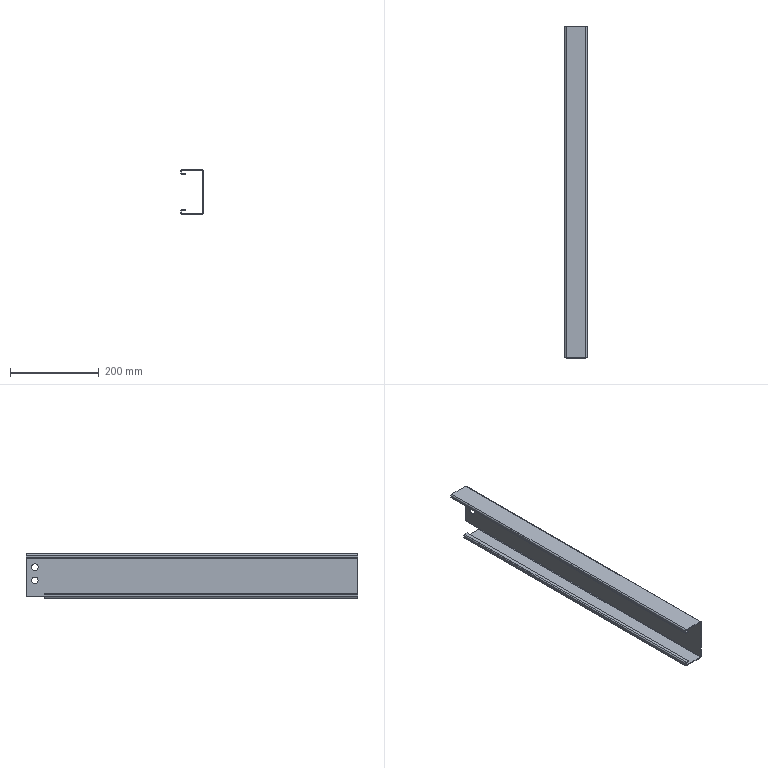Part | SolidWorks | features EdgeFlange 3, ICE 2, FlatPattern 1, SMBaseFlange 1, SheetMetal 1 | 1 solid | 60 faces | box 50 x 750 x 100 mm | volume 328411 mm3 | plane 44 | cylinder 16 | commonest cylinder face diameters 2 x4 6 x4 15 x4 1.473 x2 5.473 x2
STEP:
#1=CARTESIAN_POINT('',(-2.,355.,-2.5));
#2=VERTEX_POINT('',#1);
#3=CARTESIAN_POINT('',(-2.,355.,-17.5));
#4=VERTEX_POINT('',#3);
#5=CARTESIAN_POINT('',(-2.,355.,-10.));
#6=DIRECTION('',(1.,0.,0.));
#7=DIRECTION('',(0.,0.,-1.));
#8=AXIS2_PLACEMENT_3D('',#5,#6,#7);
#9=CIRCLE('',#8,7.5);
#10=EDGE_CURVE('',#2,#4,#9,.T.);
#11=ORIENTED_EDGE('',*,*,#10,.F.);
#12=CARTESIAN_POINT('',(0.,355.,-2.5));
#13=VERTEX_POINT('',#12);
#14=CARTESIAN_POINT('',(-10.,355.,-2.5));
#15=DIRECTION('',(1.,0.,0.));
#16=VECTOR('',#15,1000.);
#17=LINE('',#14,#16);
#18=EDGE_CURVE('',#2,#13,#17,.T.);
#19=ORIENTED_EDGE('',*,*,#18,.T.);
#20=CARTESIAN_POINT('',(0.,355.,-17.5));
#21=VERTEX_POINT('',#20);
#22=CARTESIAN_POINT('',(0.,355.,-10.));
#23=DIRECTION('',(1.,0.,0.));
#24=DIRECTION('',(0.,0.,-1.));
#25=AXIS2_PLACEMENT_3D('',#22,#23,#24);
#26=CIRCLE('',#25,7.5);
#27=EDGE_CURVE('',#13,#21,#26,.T.);
#28=ORIENTED_EDGE('',*,*,#27,.T.);
#29=CARTESIAN_POINT('',(-10.,355.,-17.5));
#30=DIRECTION('',(1.,0.,0.));
#31=VECTOR('',#30,1000.);
#32=LINE('',#29,#31);
#33=EDGE_CURVE('',#4,#21,#32,.T.);
#34=ORIENTED_EDGE('',*,*,#33,.F.);
#35=EDGE_LOOP('',(#11,#19,#28,#34));
#36=FACE_OUTER_BOUND('',#35,.T.);
#37=CARTESIAN_POINT('',(-10.,355.,-10.));
#38=DIRECTION('',(1.,0.,0.));
#39=DIRECTION('',(0.,0.,-1.));
#40=AXIS2_PLACEMENT_3D('',#37,#38,#39);
#41=CYLINDRICAL_SURFACE('',#40,7.5);
#42=ADVANCED_FACE('',(#36),#41,.F.);
#43=CARTESIAN_POINT('',(-2.,355.,27.5));
#44=VERTEX_POINT('',#43);
#45=CARTESIAN_POINT('',(-2.,355.,12.5));
#46=VERTEX_POINT('',#45);
#47=CARTESIAN_POINT('',(-2.,355.,20.));
#48=DIRECTION('',(1.,0.,0.));
#49=DIRECTION('',(0.,0.,-1.));
#50=AXIS2_PLACEMENT_3D('',#47,#48,#49);
#51=CIRCLE('',#50,7.5);
#52=EDGE_CURVE('',#44,#46,#51,.T.);
#53=ORIENTED_EDGE('',*,*,#52,.F.);
#54=CARTESIAN_POINT('',(0.,355.,27.5));
#55=VERTEX_POINT('',#54);
#56=CARTESIAN_POINT('',(-10.,355.,27.5));
#57=DIRECTION('',(1.,0.,0.));
#58=VECTOR('',#57,1000.);
#59=LINE('',#56,#58);
#60=EDGE_CURVE('',#44,#55,#59,.T.);
#61=ORIENTED_EDGE('',*,*,#60,.T.);
#62=CARTESIAN_POINT('',(0.,355.,12.5));
#63=VERTEX_POINT('',#62);
#64=CARTESIAN_POINT('',(0.,355.,20.));
#65=DIRECTION('',(1.,0.,0.));
#66=DIRECTION('',(0.,0.,-1.));
#67=AXIS2_PLACEMENT_3D('',#64,#65,#66);
#68=CIRCLE('',#67,7.5);
#69=EDGE_CURVE('',#55,#63,#68,.T.);
#70=ORIENTED_EDGE('',*,*,#69,.T.);
#71=CARTESIAN_POINT('',(-10.,355.,12.5));
#72=DIRECTION('',(1.,0.,0.));
#73=VECTOR('',#72,1000.);
#74=LINE('',#71,#73);
#75=EDGE_CURVE('',#46,#63,#74,.T.);
#76=ORIENTED_EDGE('',*,*,#75,.F.);
#77=EDGE_LOOP('',(#53,#61,#70,#76));
#78=FACE_OUTER_BOUND('',#77,.T.);
#79=CARTESIAN_POINT('',(-10.,355.,20.));
#80=DIRECTION('',(1.,0.,0.));
#81=DIRECTION('',(0.,0.,-1.));
#82=AXIS2_PLACEMENT_3D('',#79,#80,#81);
#83=CYLINDRICAL_SURFACE('',#82,7.5);
#84=ADVANCED_FACE('',(#78),#83,.F.);
#85=CARTESIAN_POINT('',(-50.,333.,-42.737));
#86=VERTEX_POINT('',#85);
#87=CARTESIAN_POINT('',(-50.,333.,-47.));
#88=VERTEX_POINT('',#87);
#89=CARTESIAN_POINT('',(-50.,333.,0.));
#90=DIRECTION('',(0.,0.,-1.));
#91=VECTOR('',#90,1000.);
#92=LINE('',#89,#91);
#93=EDGE_CURVE('',#86,#88,#92,.T.);
#94=ORIENTED_EDGE('',*,*,#93,.T.);
#95=CARTESIAN_POINT('',(-50.,-375.,-47.));
#96=VERTEX_POINT('',#95);
#97=CARTESIAN_POINT('',(-50.,375.,-47.));
#98=DIRECTION('',(0.,1.,0.));
#99=VECTOR('',#98,1000.);
#100=LINE('',#97,#99);
#101=EDGE_CURVE('',#96,#88,#100,.T.);
#102=ORIENTED_EDGE('',*,*,#101,.F.);
#103=CARTESIAN_POINT('',(-50.,-375.,-42.737));
#104=VERTEX_POINT('',#103);
#105=CARTESIAN_POINT('',(-50.,-375.,0.));
#106=DIRECTION('',(0.,0.,1.));
#107=VECTOR('',#106,1000.);
#108=LINE('',#105,#107);
#109=EDGE_CURVE('',#96,#104,#108,.T.);
#110=ORIENTED_EDGE('',*,*,#109,.T.);
#111=CARTESIAN_POINT('',(-50.,-375.,-42.737));
#112=DIRECTION('',(0.,1.,0.));
#113=VECTOR('',#112,1000.);
#114=LINE('',#111,#113);
#115=EDGE_CURVE('',#104,#86,#114,.T.);
#116=ORIENTED_EDGE('',*,*,#115,.T.);
#117=EDGE_LOOP('',(#94,#102,#110,#116));
#118=FACE_OUTER_BOUND('',#117,.T.);
#119=CARTESIAN_POINT('',(-50.,0.,0.));
#120=DIRECTION('',(1.,0.,0.));
#121=DIRECTION('',(0.,0.,-1.));
#122=AXIS2_PLACEMENT_3D('',#119,#120,#121);
#123=PLANE('',#122);
#124=ADVANCED_FACE('',(#118),#123,.F.);
#125=CARTESIAN_POINT('',(-48.,333.,-47.));
#126=VERTEX_POINT('',#125);
#127=CARTESIAN_POINT('',(-48.,-375.,-47.));
#128=VERTEX_POINT('',#127);
#129=CARTESIAN_POINT('',(-48.,375.,-47.));
#130=DIRECTION('',(0.,-1.,0.));
#131=VECTOR('',#130,1000.);
#132=LINE('',#129,#131);
#133=EDGE_CURVE('',#126,#128,#132,.T.);
#134=ORIENTED_EDGE('',*,*,#133,.F.);
#135=CARTESIAN_POINT('',(-48.,333.,-42.737));
#136=VERTEX_POINT('',#135);
#137=CARTESIAN_POINT('',(-48.,333.,0.));
#138=DIRECTION('',(0.,0.,-1.));
#139=VECTOR('',#138,1000.);
#140=LINE('',#137,#139);
#141=EDGE_CURVE('',#136,#126,#140,.T.);
#142=ORIENTED_EDGE('',*,*,#141,.F.);
#143=CARTESIAN_POINT('',(-48.,-375.,-42.737));
#144=VERTEX_POINT('',#143);
#145=CARTESIAN_POINT('',(-48.,-375.,-42.737));
#146=DIRECTION('',(0.,1.,0.));
#147=VECTOR('',#146,1000.);
#148=LINE('',#145,#147);
#149=EDGE_CURVE('',#144,#136,#148,.T.);
#150=ORIENTED_EDGE('',*,*,#149,.F.);
#151=CARTESIAN_POINT('',(-48.,-375.,-40.));
#152=DIRECTION('',(0.,0.,1.));
#153=VECTOR('',#152,1000.);
#154=LINE('',#151,#153);
#155=EDGE_CURVE('',#128,#144,#154,.T.);
#156=ORIENTED_EDGE('',*,*,#155,.F.);
#157=EDGE_LOOP('',(#134,#142,#150,#156));
#158=FACE_OUTER_BOUND('',#157,.T.);
#159=CARTESIAN_POINT('',(-48.,0.,0.));
#160=DIRECTION('',(1.,0.,0.));
#161=DIRECTION('',(0.,0.,-1.));
#162=AXIS2_PLACEMENT_3D('',#159,#160,#161);
#163=PLANE('',#162);
#164=ADVANCED_FACE('',(#158),#163,.T.);
#165=CARTESIAN_POINT('',(-47.,333.,-50.));
#166=VERTEX_POINT('',#165);
#167=CARTESIAN_POINT('',(-3.,333.,-50.));
#168=VERTEX_POINT('',#167);
#169=CARTESIAN_POINT('',(0.,333.,-50.));
#170=DIRECTION('',(1.,0.,0.));
#171=VECTOR('',#170,1000.);
#172=LINE('',#169,#171);
#173=EDGE_CURVE('',#166,#168,#172,.T.);
#174=ORIENTED_EDGE('',*,*,#173,.T.);
#175=CARTESIAN_POINT('',(-3.,-375.,-50.));
#176=VERTEX_POINT('',#175);
#177=CARTESIAN_POINT('',(-3.,375.,-50.));
#178=DIRECTION('',(0.,1.,0.));
#179=VECTOR('',#178,1000.);
#180=LINE('',#177,#179);
#181=EDGE_CURVE('',#176,#168,#180,.T.);
#182=ORIENTED_EDGE('',*,*,#181,.F.);
#183=CARTESIAN_POINT('',(-47.,-375.,-50.));
#184=VERTEX_POINT('',#183);
#185=CARTESIAN_POINT('',(-50.,-375.,-50.));
#186=DIRECTION('',(1.,0.,0.));
#187=VECTOR('',#186,1000.);
#188=LINE('',#185,#187);
#189=EDGE_CURVE('',#184,#176,#188,.T.);
#190=ORIENTED_EDGE('',*,*,#189,.F.);
#191=CARTESIAN_POINT('',(-47.,-375.,-50.));
#192=DIRECTION('',(0.,1.,0.));
#193=VECTOR('',#192,1000.);
#194=LINE('',#191,#193);
#195=EDGE_CURVE('',#184,#166,#194,.T.);
#196=ORIENTED_EDGE('',*,*,#195,.T.);
#197=EDGE_LOOP('',(#174,#182,#190,#196));
#198=FACE_OUTER_BOUND('',#197,.T.);
#199=CARTESIAN_POINT('',(0.,0.,-50.));
#200=DIRECTION('',(0.,0.,1.));
#201=DIRECTION('',(1.,0.,0.));
#202=AXIS2_PLACEMENT_3D('',#199,#200,#201);
#203=PLANE('',#202);
#204=ADVANCED_FACE('',(#198),#203,.F.);
#205=CARTESIAN_POINT('',(-3.,333.,-48.));
#206=VERTEX_POINT('',#205);
#207=CARTESIAN_POINT('',(-3.,-375.,-48.));
#208=VERTEX_POINT('',#207);
#209=CARTESIAN_POINT('',(-3.,375.,-48.));
#210=DIRECTION('',(0.,-1.,0.));
#211=VECTOR('',#210,1000.);
#212=LINE('',#209,#211);
#213=EDGE_CURVE('',#206,#208,#212,.T.);
#214=ORIENTED_EDGE('',*,*,#213,.F.);
#215=CARTESIAN_POINT('',(-47.,333.,-48.));
#216=VERTEX_POINT('',#215);
#217=CARTESIAN_POINT('',(0.,333.,-48.));
#218=DIRECTION('',(1.,0.,0.));
#219=VECTOR('',#218,1000.);
#220=LINE('',#217,#219);
#221=EDGE_CURVE('',#216,#206,#220,.T.);
#222=ORIENTED_EDGE('',*,*,#221,.F.);
#223=CARTESIAN_POINT('',(-47.,-375.,-48.));
#224=VERTEX_POINT('',#223);
#225=CARTESIAN_POINT('',(-47.,-375.,-48.));
#226=DIRECTION('',(0.,1.,0.));
#227=VECTOR('',#226,1000.);
#228=LINE('',#225,#227);
#229=EDGE_CURVE('',#224,#216,#228,.T.);
#230=ORIENTED_EDGE('',*,*,#229,.F.);
#231=CARTESIAN_POINT('',(0.,-375.,-48.));
#232=DIRECTION('',(1.,0.,0.));
#233=VECTOR('',#232,1000.);
#234=LINE('',#231,#233);
#235=EDGE_CURVE('',#224,#208,#234,.T.);
#236=ORIENTED_EDGE('',*,*,#235,.T.);
#237=EDGE_LOOP('',(#214,#222,#230,#236));
#238=FACE_OUTER_BOUND('',#237,.T.);
#239=CARTESIAN_POINT('',(0.,0.,-48.));
#240=DIRECTION('',(0.,0.,1.));
#241=DIRECTION('',(1.,0.,0.));
#242=AXIS2_PLACEMENT_3D('',#239,#240,#241);
#243=PLANE('',#242);
#244=ADVANCED_FACE('',(#238),#243,.T.);
#245=CARTESIAN_POINT('',(-2.,355.,-10.));
#246=DIRECTION('',(1.,0.,0.));
#247=DIRECTION('',(0.,0.,-1.));
#248=AXIS2_PLACEMENT_3D('',#245,#246,#247);
#249=CIRCLE('',#248,7.5);
#250=EDGE_CURVE('',#4,#2,#249,.T.);
#251=ORIENTED_EDGE('',*,*,#250,.T.);
#252=ORIENTED_EDGE('',*,*,#10,.T.);
#253=EDGE_LOOP('',(#251,#252));
#254=FACE_BOUND('',#253,.T.);
#255=CARTESIAN_POINT('',(-2.,355.,20.));
#256=DIRECTION('',(1.,0.,0.));
#257=DIRECTION('',(0.,0.,-1.));
#258=AXIS2_PLACEMENT_3D('',#255,#256,#257);
#259=CIRCLE('',#258,7.5);
#260=EDGE_CURVE('',#46,#44,#259,.T.);
#261=ORIENTED_EDGE('',*,*,#260,.T.);
#262=ORIENTED_EDGE('',*,*,#52,.T.);
#263=EDGE_LOOP('',(#261,#262));
#264=FACE_BOUND('',#263,.T.);
#265=CARTESIAN_POINT('',(-2.,333.,-46.112));
#266=VERTEX_POINT('',#265);
#267=CARTESIAN_POINT('',(-2.,333.,-47.));
#268=VERTEX_POINT('',#267);
#269=CARTESIAN_POINT('',(-2.,333.,0.));
#270=DIRECTION('',(0.,0.,-1.));
#271=VECTOR('',#270,1000.);
#272=LINE('',#269,#271);
#273=EDGE_CURVE('',#266,#268,#272,.T.);
#274=ORIENTED_EDGE('',*,*,#273,.T.);
#275=CARTESIAN_POINT('',(-2.,-375.,-47.));
#276=VERTEX_POINT('',#275);
#277=CARTESIAN_POINT('',(-2.,-375.,-47.));
#278=DIRECTION('',(0.,1.,0.));
#279=VECTOR('',#278,1000.);
#280=LINE('',#277,#279);
#281=EDGE_CURVE('',#276,#268,#280,.T.);
#282=ORIENTED_EDGE('',*,*,#281,.F.);
#283=CARTESIAN_POINT('',(-2.,-375.,47.));
#284=VERTEX_POINT('',#283);
#285=CARTESIAN_POINT('',(-2.,-375.,50.));
#286=DIRECTION('',(0.,0.,-1.));
#287=VECTOR('',#286,1000.);
#288=LINE('',#285,#287);
#289=EDGE_CURVE('',#284,#276,#288,.T.);
#290=ORIENTED_EDGE('',*,*,#289,.F.);
#291=CARTESIAN_POINT('',(-2.,375.,47.));
#292=VERTEX_POINT('',#291);
#293=CARTESIAN_POINT('',(-2.,375.,47.));
#294=DIRECTION('',(0.,-1.,0.));
#295=VECTOR('',#294,1000.);
#296=LINE('',#293,#295);
#297=EDGE_CURVE('',#292,#284,#296,.T.);
#298=ORIENTED_EDGE('',*,*,#297,.F.);
#299=CARTESIAN_POINT('',(-2.,375.,-46.112));
#300=VERTEX_POINT('',#299);
#301=CARTESIAN_POINT('',(-2.,375.,50.));
#302=DIRECTION('',(0.,0.,1.));
#303=VECTOR('',#302,1000.);
#304=LINE('',#301,#303);
#305=EDGE_CURVE('',#300,#292,#304,.T.);
#306=ORIENTED_EDGE('',*,*,#305,.F.);
#307=CARTESIAN_POINT('',(-2.,0.,-46.112));
#308=DIRECTION('',(0.,-1.,0.));
#309=VECTOR('',#308,1000.);
#310=LINE('',#307,#309);
#311=EDGE_CURVE('',#300,#266,#310,.T.);
#312=ORIENTED_EDGE('',*,*,#311,.T.);
#313=EDGE_LOOP('',(#274,#282,#290,#298,#306,#312));
#314=FACE_OUTER_BOUND('',#313,.T.);
#315=CARTESIAN_POINT('',(-2.,0.,0.));
#316=DIRECTION('',(1.,0.,0.));
#317=DIRECTION('',(0.,0.,-1.));
#318=AXIS2_PLACEMENT_3D('',#315,#316,#317);
#319=PLANE('',#318);
#320=ADVANCED_FACE('',(#254,#264,#314),#319,.F.);
#321=CARTESIAN_POINT('',(0.,355.,-10.));
#322=DIRECTION('',(1.,0.,0.));
#323=DIRECTION('',(0.,0.,-1.));
#324=AXIS2_PLACEMENT_3D('',#321,#322,#323);
#325=CIRCLE('',#324,7.5);
#326=EDGE_CURVE('',#21,#13,#325,.T.);
#327=ORIENTED_EDGE('',*,*,#326,.F.);
#328=ORIENTED_EDGE('',*,*,#27,.F.);
#329=EDGE_LOOP('',(#327,#328));
#330=FACE_BOUND('',#329,.T.);
#331=CARTESIAN_POINT('',(0.,355.,20.));
#332=DIRECTION('',(1.,0.,0.));
#333=DIRECTION('',(0.,0.,-1.));
#334=AXIS2_PLACEMENT_3D('',#331,#332,#333);
#335=CIRCLE('',#334,7.5);
#336=EDGE_CURVE('',#63,#55,#335,.T.);
#337=ORIENTED_EDGE('',*,*,#336,.F.);
#338=ORIENTED_EDGE('',*,*,#69,.F.);
#339=EDGE_LOOP('',(#337,#338));
#340=FACE_BOUND('',#339,.T.);
#341=CARTESIAN_POINT('',(0.,-375.,-47.));
#342=VERTEX_POINT('',#341);
#343=CARTESIAN_POINT('',(0.,333.,-47.));
#344=VERTEX_POINT('',#343);
#345=CARTESIAN_POINT('',(0.,-375.,-47.));
#346=DIRECTION('',(0.,1.,0.));
#347=VECTOR('',#346,1000.);
#348=LINE('',#345,#347);
#349=EDGE_CURVE('',#342,#344,#348,.T.);
#350=ORIENTED_EDGE('',*,*,#349,.T.);
#351=CARTESIAN_POINT('',(0.,333.,-46.112));
#352=VERTEX_POINT('',#351);
#353=CARTESIAN_POINT('',(0.,333.,0.));
#354=DIRECTION('',(0.,0.,-1.));
#355=VECTOR('',#354,1000.);
#356=LINE('',#353,#355);
#357=EDGE_CURVE('',#352,#344,#356,.T.);
#358=ORIENTED_EDGE('',*,*,#357,.F.);
#359=CARTESIAN_POINT('',(0.,375.,-46.112));
#360=VERTEX_POINT('',#359);
#361=CARTESIAN_POINT('',(0.,0.,-46.112));
#362=DIRECTION('',(0.,-1.,0.));
#363=VECTOR('',#362,1000.);
#364=LINE('',#361,#363);
#365=EDGE_CURVE('',#360,#352,#364,.T.);
#366=ORIENTED_EDGE('',*,*,#365,.F.);
#367=CARTESIAN_POINT('',(0.,375.,47.));
#368=VERTEX_POINT('',#367);
#369=CARTESIAN_POINT('',(0.,375.,50.));
#370=DIRECTION('',(0.,0.,1.));
#371=VECTOR('',#370,1000.);
#372=LINE('',#369,#371);
#373=EDGE_CURVE('',#360,#368,#372,.T.);
#374=ORIENTED_EDGE('',*,*,#373,.T.);
#375=CARTESIAN_POINT('',(0.,-375.,47.));
#376=VERTEX_POINT('',#375);
#377=CARTESIAN_POINT('',(0.,375.,47.));
#378=DIRECTION('',(0.,-1.,0.));
#379=VECTOR('',#378,1000.);
#380=LINE('',#377,#379);
#381=EDGE_CURVE('',#368,#376,#380,.T.);
#382=ORIENTED_EDGE('',*,*,#381,.T.);
#383=CARTESIAN_POINT('',(0.,-375.,50.));
#384=DIRECTION('',(0.,0.,-1.));
#385=VECTOR('',#384,1000.);
#386=LINE('',#383,#385);
#387=EDGE_CURVE('',#376,#342,#386,.T.);
#388=ORIENTED_EDGE('',*,*,#387,.T.);
#389=EDGE_LOOP('',(#350,#358,#366,#374,#382,#388));
#390=FACE_OUTER_BOUND('',#389,.T.);
#391=CARTESIAN_POINT('',(0.,0.,0.));
#392=DIRECTION('',(1.,0.,0.));
#393=DIRECTION('',(0.,0.,-1.));
#394=AXIS2_PLACEMENT_3D('',#391,#392,#393);
#395=PLANE('',#394);
#396=ADVANCED_FACE('',(#330,#340,#390),#395,.T.);
#397=ORIENTED_EDGE('',*,*,#373,.F.);
#398=CARTESIAN_POINT('',(-2.,375.,-46.112));
#399=DIRECTION('',(1.,0.,0.));
#400=VECTOR('',#399,1000.);
#401=LINE('',#398,#400);
#402=EDGE_CURVE('',#300,#360,#401,.T.);
#403=ORIENTED_EDGE('',*,*,#402,.F.);
#404=ORIENTED_EDGE('',*,*,#305,.T.);
#405=CARTESIAN_POINT('',(-2.,375.,47.));
#406=DIRECTION('',(1.,0.,0.));
#407=VECTOR('',#406,1000.);
#408=LINE('',#405,#407);
#409=EDGE_CURVE('',#292,#368,#408,.T.);
#410=ORIENTED_EDGE('',*,*,#409,.T.);
#411=EDGE_LOOP('',(#397,#403,#404,#410));
#412=FACE_OUTER_BOUND('',#411,.T.);
#413=CARTESIAN_POINT('',(-2.,375.,50.));
#414=DIRECTION('',(0.,1.,0.));
#415=DIRECTION('',(0.,0.,1.));
#416=AXIS2_PLACEMENT_3D('',#413,#414,#415);
#417=PLANE('',#416);
#418=ADVANCED_FACE('',(#412),#417,.T.);
#419=ORIENTED_EDGE('',*,*,#181,.T.);
#420=CARTESIAN_POINT('',(-3.,333.,-47.));
#421=DIRECTION('',(0.,1.,0.));
#422=DIRECTION('',(0.,0.,-1.));
#423=AXIS2_PLACEMENT_3D('',#420,#421,#422);
#424=CIRCLE('',#423,3.);
#425=EDGE_CURVE('',#344,#168,#424,.T.);
#426=ORIENTED_EDGE('',*,*,#425,.F.);
#427=ORIENTED_EDGE('',*,*,#349,.F.);
#428=CARTESIAN_POINT('',(-3.,-375.,-47.));
#429=DIRECTION('',(0.,-1.,0.));
#430=DIRECTION('',(0.,0.,-1.));
#431=AXIS2_PLACEMENT_3D('',#428,#429,#430);
#432=CIRCLE('',#431,3.);
#433=EDGE_CURVE('',#176,#342,#432,.T.);
#434=ORIENTED_EDGE('',*,*,#433,.F.);
#435=EDGE_LOOP('',(#419,#426,#427,#434));
#436=FACE_OUTER_BOUND('',#435,.T.);
#437=CARTESIAN_POINT('',(-3.,-375.,-47.));
#438=DIRECTION('',(0.,-1.,0.));
#439=DIRECTION('',(0.,0.,-1.));
#440=AXIS2_PLACEMENT_3D('',#437,#438,#439);
#441=CYLINDRICAL_SURFACE('',#440,3.);
#442=ADVANCED_FACE('',(#436),#441,.T.);
#443=CARTESIAN_POINT('',(-3.,333.,-47.));
#444=DIRECTION('',(0.,1.,0.));
#445=DIRECTION('',(0.,0.,-1.));
#446=AXIS2_PLACEMENT_3D('',#443,#444,#445);
#447=CIRCLE('',#446,1.);
#448=EDGE_CURVE('',#268,#206,#447,.T.);
#449=ORIENTED_EDGE('',*,*,#448,.T.);
#450=ORIENTED_EDGE('',*,*,#213,.T.);
#451=CARTESIAN_POINT('',(-3.,-375.,-47.));
#452=DIRECTION('',(0.,-1.,0.));
#453=DIRECTION('',(0.,0.,-1.));
#454=AXIS2_PLACEMENT_3D('',#451,#452,#453);
#455=CIRCLE('',#454,1.);
#456=EDGE_CURVE('',#208,#276,#455,.T.);
#457=ORIENTED_EDGE('',*,*,#456,.T.);
#458=ORIENTED_EDGE('',*,*,#281,.T.);
#459=EDGE_LOOP('',(#449,#450,#457,#458));
#460=FACE_OUTER_BOUND('',#459,.T.);
#461=CARTESIAN_POINT('',(-3.,-375.,-47.));
#462=DIRECTION('',(0.,-1.,0.));
#463=DIRECTION('',(0.,0.,-1.));
#464=AXIS2_PLACEMENT_3D('',#461,#462,#463);
#465=CYLINDRICAL_SURFACE('',#464,1.);
#466=ADVANCED_FACE('',(#460),#465,.F.);
#467=ORIENTED_EDGE('',*,*,#101,.T.);
#468=CARTESIAN_POINT('',(-47.,333.,-47.));
#469=DIRECTION('',(0.,1.,0.));
#470=DIRECTION('',(0.,0.,-1.));
#471=AXIS2_PLACEMENT_3D('',#468,#469,#470);
#472=CIRCLE('',#471,3.);
#473=EDGE_CURVE('',#166,#88,#472,.T.);
#474=ORIENTED_EDGE('',*,*,#473,.F.);
#475=ORIENTED_EDGE('',*,*,#195,.F.);
#476=CARTESIAN_POINT('',(-47.,-375.,-47.));
#477=DIRECTION('',(0.,-1.,0.));
#478=DIRECTION('',(0.,0.,-1.));
#479=AXIS2_PLACEMENT_3D('',#476,#477,#478);
#480=CIRCLE('',#479,3.);
#481=EDGE_CURVE('',#96,#184,#480,.T.);
#482=ORIENTED_EDGE('',*,*,#481,.F.);
#483=EDGE_LOOP('',(#467,#474,#475,#482));
#484=FACE_OUTER_BOUND('',#483,.T.);
#485=CARTESIAN_POINT('',(-47.,-375.,-47.));
#486=DIRECTION('',(0.,-1.,0.));
#487=DIRECTION('',(-1.,0.,0.));
#488=AXIS2_PLACEMENT_3D('',#485,#486,#487);
#489=CYLINDRICAL_SURFACE('',#488,3.);
#490=ADVANCED_FACE('',(#484),#489,.T.);
#491=CARTESIAN_POINT('',(-47.,333.,-47.));
#492=DIRECTION('',(0.,1.,0.));
#493=DIRECTION('',(0.,0.,-1.));
#494=AXIS2_PLACEMENT_3D('',#491,#492,#493);
#495=CIRCLE('',#494,1.);
#496=EDGE_CURVE('',#216,#126,#495,.T.);
#497=ORIENTED_EDGE('',*,*,#496,.T.);
#498=ORIENTED_EDGE('',*,*,#133,.T.);
#499=CARTESIAN_POINT('',(-47.,-375.,-47.));
#500=DIRECTION('',(0.,-1.,0.));
#501=DIRECTION('',(0.,0.,-1.));
#502=AXIS2_PLACEMENT_3D('',#499,#500,#501);
#503=CIRCLE('',#502,1.);
#504=EDGE_CURVE('',#128,#224,#503,.T.);
#505=ORIENTED_EDGE('',*,*,#504,.T.);
#506=ORIENTED_EDGE('',*,*,#229,.T.);
#507=EDGE_LOOP('',(#497,#498,#505,#506));
#508=FACE_OUTER_BOUND('',#507,.T.);
#509=CARTESIAN_POINT('',(-47.,-375.,-47.));
#510=DIRECTION('',(0.,-1.,0.));
#511=DIRECTION('',(-1.,0.,0.));
#512=AXIS2_PLACEMENT_3D('',#509,#510,#511);
#513=CYLINDRICAL_SURFACE('',#512,1.);
#514=ADVANCED_FACE('',(#508),#513,.F.);
#515=CARTESIAN_POINT('',(-47.263,333.,-40.));
#516=VERTEX_POINT('',#515);
#517=CARTESIAN_POINT('',(-47.263,-375.,-40.));
#518=VERTEX_POINT('',#517);
#519=CARTESIAN_POINT('',(-47.263,0.,-40.));
#520=DIRECTION('',(0.,-1.,0.));
#521=VECTOR('',#520,1000.);
#522=LINE('',#519,#521);
#523=EDGE_CURVE('',#516,#518,#522,.T.);
#524=ORIENTED_EDGE('',*,*,#523,.F.);
#525=CARTESIAN_POINT('',(-47.263,333.,-42.737));
#526=DIRECTION('',(0.,1.,0.));
#527=DIRECTION('',(0.,0.,-1.));
#528=AXIS2_PLACEMENT_3D('',#525,#526,#527);
#529=CIRCLE('',#528,2.737);
#530=EDGE_CURVE('',#86,#516,#529,.T.);
#531=ORIENTED_EDGE('',*,*,#530,.F.);
#532=ORIENTED_EDGE('',*,*,#115,.F.);
#533=CARTESIAN_POINT('',(-47.263,-375.,-42.737));
#534=DIRECTION('',(0.,-1.,0.));
#535=DIRECTION('',(0.,0.,-1.));
#536=AXIS2_PLACEMENT_3D('',#533,#534,#535);
#537=CIRCLE('',#536,2.737);
#538=EDGE_CURVE('',#518,#104,#537,.T.);
#539=ORIENTED_EDGE('',*,*,#538,.F.);
#540=EDGE_LOOP('',(#524,#531,#532,#539));
#541=FACE_OUTER_BOUND('',#540,.T.);
#542=CARTESIAN_POINT('',(-47.263,-375.,-42.737));
#543=DIRECTION('',(0.,-1.,0.));
#544=DIRECTION('',(0.,0.,1.));
#545=AXIS2_PLACEMENT_3D('',#542,#543,#544);
#546=CYLINDRICAL_SURFACE('',#545,2.737);
#547=ADVANCED_FACE('',(#541),#546,.T.);
#548=CARTESIAN_POINT('',(-47.263,333.,-42.));
#549=VERTEX_POINT('',#548);
#550=CARTESIAN_POINT('',(-47.263,333.,-42.737));
#551=DIRECTION('',(0.,1.,0.));
#552=DIRECTION('',(0.,0.,-1.));
#553=AXIS2_PLACEMENT_3D('',#550,#551,#552);
#554=CIRCLE('',#553,0.7366);
#555=EDGE_CURVE('',#136,#549,#554,.T.);
#556=ORIENTED_EDGE('',*,*,#555,.T.);
#557=CARTESIAN_POINT('',(-47.263,-375.,-42.));
#558=VERTEX_POINT('',#557);
#559=CARTESIAN_POINT('',(-47.263,375.,-42.));
#560=DIRECTION('',(0.,-1.,0.));
#561=VECTOR('',#560,1000.);
#562=LINE('',#559,#561);
#563=EDGE_CURVE('',#549,#558,#562,.T.);
#564=ORIENTED_EDGE('',*,*,#563,.T.);
#565=CARTESIAN_POINT('',(-47.263,-375.,-42.737));
#566=DIRECTION('',(0.,-1.,0.));
#567=DIRECTION('',(0.,0.,-1.));
#568=AXIS2_PLACEMENT_3D('',#565,#566,#567);
#569=CIRCLE('',#568,0.7366);
#570=EDGE_CURVE('',#558,#144,#569,.T.);
#571=ORIENTED_EDGE('',*,*,#570,.T.);
#572=ORIENTED_EDGE('',*,*,#149,.T.);
#573=EDGE_LOOP('',(#556,#564,#571,#572));
#574=FACE_OUTER_BOUND('',#573,.T.);
#575=CARTESIAN_POINT('',(-47.263,-375.,-42.737));
#576=DIRECTION('',(0.,-1.,0.));
#577=DIRECTION('',(0.,0.,1.));
#578=AXIS2_PLACEMENT_3D('',#575,#576,#577);
#579=CYLINDRICAL_SURFACE('',#578,0.7366);
#580=ADVANCED_FACE('',(#574),#579,.F.);
#581=CARTESIAN_POINT('',(-40.,333.,-40.));
#582=VERTEX_POINT('',#581);
#583=CARTESIAN_POINT('',(-40.,-375.,-40.));
#584=VERTEX_POINT('',#583);
#585=CARTESIAN_POINT('',(-40.,-375.,-40.));
#586=DIRECTION('',(0.,-1.,0.));
#587=VECTOR('',#586,1000.);
#588=LINE('',#585,#587);
#589=EDGE_CURVE('',#582,#584,#588,.T.);
#590=ORIENTED_EDGE('',*,*,#589,.F.);
#591=CARTESIAN_POINT('',(0.,333.,-40.));
#592=DIRECTION('',(1.,0.,0.));
#593=VECTOR('',#592,1000.);
#594=LINE('',#591,#593);
#595=EDGE_CURVE('',#516,#582,#594,.T.);
#596=ORIENTED_EDGE('',*,*,#595,.F.);
#597=ORIENTED_EDGE('',*,*,#523,.T.);
#598=CARTESIAN_POINT('',(-48.,-375.,-40.));
#599=DIRECTION('',(-1.,0.,0.));
#600=VECTOR('',#599,1000.);
#601=LINE('',#598,#600);
#602=EDGE_CURVE('',#584,#518,#601,.T.);
#603=ORIENTED_EDGE('',*,*,#602,.F.);
#604=EDGE_LOOP('',(#590,#596,#597,#603));
#605=FACE_OUTER_BOUND('',#604,.T.);
#606=CARTESIAN_POINT('',(0.,0.,-40.));
#607=DIRECTION('',(0.,0.,1.));
#608=DIRECTION('',(1.,0.,0.));
#609=AXIS2_PLACEMENT_3D('',#606,#607,#608);
#610=PLANE('',#609);
#611=ADVANCED_FACE('',(#605),#610,.T.);
#612=CARTESIAN_POINT('',(-40.,333.,-42.));
#613=VERTEX_POINT('',#612);
#614=CARTESIAN_POINT('',(0.,333.,-42.));
#615=DIRECTION('',(1.,0.,0.));
#616=VECTOR('',#615,1000.);
#617=LINE('',#614,#616);
#618=EDGE_CURVE('',#549,#613,#617,.T.);
#619=ORIENTED_EDGE('',*,*,#618,.T.);
#620=CARTESIAN_POINT('',(-40.,-375.,-42.));
#621=VERTEX_POINT('',#620);
#622=CARTESIAN_POINT('',(-40.,0.,-42.));
#623=DIRECTION('',(0.,-1.,0.));
#624=VECTOR('',#623,1000.);
#625=LINE('',#622,#624);
#626=EDGE_CURVE('',#613,#621,#625,.T.);
#627=ORIENTED_EDGE('',*,*,#626,.T.);
#628=CARTESIAN_POINT('',(0.,-375.,-42.));
#629=DIRECTION('',(-1.,0.,0.));
#630=VECTOR('',#629,1000.);
#631=LINE('',#628,#630);
#632=EDGE_CURVE('',#621,#558,#631,.T.);
#633=ORIENTED_EDGE('',*,*,#632,.T.);
#634=ORIENTED_EDGE('',*,*,#563,.F.);
#635=EDGE_LOOP('',(#619,#627,#633,#634));
#636=FACE_OUTER_BOUND('',#635,.T.);
#637=CARTESIAN_POINT('',(0.,0.,-42.));
#638=DIRECTION('',(0.,0.,1.));
#639=DIRECTION('',(1.,0.,0.));
#640=AXIS2_PLACEMENT_3D('',#637,#638,#639);
#641=PLANE('',#640);
#642=ADVANCED_FACE('',(#636),#641,.F.);
#643=ORIENTED_EDGE('',*,*,#626,.F.);
#644=CARTESIAN_POINT('',(-40.,333.,-42.));
#645=DIRECTION('',(0.,0.,1.));
#646=VECTOR('',#645,1000.);
#647=LINE('',#644,#646);
#648=EDGE_CURVE('',#613,#582,#647,.T.);
#649=ORIENTED_EDGE('',*,*,#648,.T.);
#650=ORIENTED_EDGE('',*,*,#589,.T.);
#651=CARTESIAN_POINT('',(-40.,-375.,-40.));
#652=DIRECTION('',(0.,0.,-1.));
#653=VECTOR('',#652,1000.);
#654=LINE('',#651,#653);
#655=EDGE_CURVE('',#584,#621,#654,.T.);
#656=ORIENTED_EDGE('',*,*,#655,.T.);
#657=EDGE_LOOP('',(#643,#649,#650,#656));
#658=FACE_OUTER_BOUND('',#657,.T.);
#659=CARTESIAN_POINT('',(-40.,-375.,-40.));
#660=DIRECTION('',(1.,0.,0.));
#661=DIRECTION('',(0.,0.,-1.));
#662=AXIS2_PLACEMENT_3D('',#659,#660,#661);
#663=PLANE('',#662);
#664=ADVANCED_FACE('',(#658),#663,.T.);
#665=CARTESIAN_POINT('',(-48.,-375.,42.737));
#666=VERTEX_POINT('',#665);
#667=CARTESIAN_POINT('',(-50.,-375.,42.737));
#668=VERTEX_POINT('',#667);
#669=CARTESIAN_POINT('',(-48.,-375.,42.737));
#670=DIRECTION('',(-1.,0.,0.));
#671=VECTOR('',#670,1000.);
#672=LINE('',#669,#671);
#673=EDGE_CURVE('',#666,#668,#672,.T.);
#674=ORIENTED_EDGE('',*,*,#673,.F.);
#675=CARTESIAN_POINT('',(-48.,-375.,47.));
#676=VERTEX_POINT('',#675);
#677=CARTESIAN_POINT('',(-48.,-375.,48.));
#678=DIRECTION('',(0.,0.,1.));
#679=VECTOR('',#678,1000.);
#680=LINE('',#677,#679);
#681=EDGE_CURVE('',#666,#676,#680,.T.);
#682=ORIENTED_EDGE('',*,*,#681,.T.);
#683=CARTESIAN_POINT('',(-50.,-375.,47.));
#684=VERTEX_POINT('',#683);
#685=CARTESIAN_POINT('',(-50.,-375.,47.));
#686=DIRECTION('',(-1.,0.,0.));
#687=VECTOR('',#686,1000.);
#688=LINE('',#685,#687);
#689=EDGE_CURVE('',#676,#684,#688,.T.);
#690=ORIENTED_EDGE('',*,*,#689,.T.);
#691=CARTESIAN_POINT('',(-50.,-375.,0.));
#692=DIRECTION('',(0.,0.,1.));
#693=VECTOR('',#692,1000.);
#694=LINE('',#691,#693);
#695=EDGE_CURVE('',#668,#684,#694,.T.);
#696=ORIENTED_EDGE('',*,*,#695,.F.);
#697=EDGE_LOOP('',(#674,#682,#690,#696));
#698=FACE_OUTER_BOUND('',#697,.T.);
#699=CARTESIAN_POINT('',(-50.,-375.,48.));
#700=DIRECTION('',(0.,1.,0.));
#701=DIRECTION('',(-1.,0.,0.));
#702=AXIS2_PLACEMENT_3D('',#699,#700,#701);
#703=PLANE('',#702);
#704=ADVANCED_FACE('',(#698),#703,.F.);
#705=CARTESIAN_POINT('',(-48.,375.,42.737));
#706=VERTEX_POINT('',#705);
#707=CARTESIAN_POINT('',(-50.,375.,42.737));
#708=VERTEX_POINT('',#707);
#709=CARTESIAN_POINT('',(-48.,375.,42.737));
#710=DIRECTION('',(-1.,0.,0.));
#711=VECTOR('',#710,1000.);
#712=LINE('',#709,#711);
#713=EDGE_CURVE('',#706,#708,#712,.T.);
#714=ORIENTED_EDGE('',*,*,#713,.T.);
#715=CARTESIAN_POINT('',(-50.,375.,47.));
#716=VERTEX_POINT('',#715);
#717=CARTESIAN_POINT('',(-50.,375.,0.));
#718=DIRECTION('',(0.,0.,-1.));
#719=VECTOR('',#718,1000.);
#720=LINE('',#717,#719);
#721=EDGE_CURVE('',#716,#708,#720,.T.);
#722=ORIENTED_EDGE('',*,*,#721,.F.);
#723=CARTESIAN_POINT('',(-48.,375.,47.));
#724=VERTEX_POINT('',#723);
#725=CARTESIAN_POINT('',(-48.,375.,47.));
#726=DIRECTION('',(-1.,0.,0.));
#727=VECTOR('',#726,1000.);
#728=LINE('',#725,#727);
#729=EDGE_CURVE('',#724,#716,#728,.T.);
#730=ORIENTED_EDGE('',*,*,#729,.F.);
#731=CARTESIAN_POINT('',(-48.,375.,40.));
#732=DIRECTION('',(0.,0.,-1.));
#733=VECTOR('',#732,1000.);
#734=LINE('',#731,#733);
#735=EDGE_CURVE('',#724,#706,#734,.T.);
#736=ORIENTED_EDGE('',*,*,#735,.T.);
#737=EDGE_LOOP('',(#714,#722,#730,#736));
#738=FACE_OUTER_BOUND('',#737,.T.);
#739=CARTESIAN_POINT('',(-50.,375.,40.));
#740=DIRECTION('',(0.,-1.,0.));
#741=DIRECTION('',(1.,0.,0.));
#742=AXIS2_PLACEMENT_3D('',#739,#740,#741);
#743=PLANE('',#742);
#744=ADVANCED_FACE('',(#738),#743,.F.);
#745=CARTESIAN_POINT('',(-50.,375.,42.737));
#746=DIRECTION('',(0.,-1.,0.));
#747=VECTOR('',#746,1000.);
#748=LINE('',#745,#747);
#749=EDGE_CURVE('',#708,#668,#748,.T.);
#750=ORIENTED_EDGE('',*,*,#749,.T.);
#751=ORIENTED_EDGE('',*,*,#695,.T.);
#752=CARTESIAN_POINT('',(-50.,-375.,47.));
#753=DIRECTION('',(0.,-1.,0.));
#754=VECTOR('',#753,1000.);
#755=LINE('',#752,#754);
#756=EDGE_CURVE('',#716,#684,#755,.T.);
#757=ORIENTED_EDGE('',*,*,#756,.F.);
#758=ORIENTED_EDGE('',*,*,#721,.T.);
#759=EDGE_LOOP('',(#750,#751,#757,#758));
#760=FACE_OUTER_BOUND('',#759,.T.);
#761=CARTESIAN_POINT('',(-50.,0.,0.));
#762=DIRECTION('',(1.,0.,0.));
#763=DIRECTION('',(0.,0.,-1.));
#764=AXIS2_PLACEMENT_3D('',#761,#762,#763);
#765=PLANE('',#764);
#766=ADVANCED_FACE('',(#760),#765,.F.);
#767=ORIENTED_EDGE('',*,*,#681,.F.);
#768=CARTESIAN_POINT('',(-48.,375.,42.737));
#769=DIRECTION('',(0.,-1.,0.));
#770=VECTOR('',#769,1000.);
#771=LINE('',#768,#770);
#772=EDGE_CURVE('',#706,#666,#771,.T.);
#773=ORIENTED_EDGE('',*,*,#772,.F.);
#774=ORIENTED_EDGE('',*,*,#735,.F.);
#775=CARTESIAN_POINT('',(-48.,-375.,47.));
#776=DIRECTION('',(0.,1.,0.));
#777=VECTOR('',#776,1000.);
#778=LINE('',#775,#777);
#779=EDGE_CURVE('',#676,#724,#778,.T.);
#780=ORIENTED_EDGE('',*,*,#779,.F.);
#781=EDGE_LOOP('',(#767,#773,#774,#780));
#782=FACE_OUTER_BOUND('',#781,.T.);
#783=CARTESIAN_POINT('',(-48.,0.,0.));
#784=DIRECTION('',(1.,0.,0.));
#785=DIRECTION('',(0.,0.,-1.));
#786=AXIS2_PLACEMENT_3D('',#783,#784,#785);
#787=PLANE('',#786);
#788=ADVANCED_FACE('',(#782),#787,.T.);
#789=CARTESIAN_POINT('',(-48.,-375.,-42.737));
#790=DIRECTION('',(-1.,0.,0.));
#791=VECTOR('',#790,1000.);
#792=LINE('',#789,#791);
#793=EDGE_CURVE('',#144,#104,#792,.T.);
#794=ORIENTED_EDGE('',*,*,#793,.T.);
#795=ORIENTED_EDGE('',*,*,#109,.F.);
#796=CARTESIAN_POINT('',(-48.,-375.,-47.));
#797=DIRECTION('',(-1.,0.,0.));
#798=VECTOR('',#797,1000.);
#799=LINE('',#796,#798);
#800=EDGE_CURVE('',#128,#96,#799,.T.);
#801=ORIENTED_EDGE('',*,*,#800,.F.);
#802=ORIENTED_EDGE('',*,*,#155,.T.);
#803=EDGE_LOOP('',(#794,#795,#801,#802));
#804=FACE_OUTER_BOUND('',#803,.T.);
#805=CARTESIAN_POINT('',(-50.,-375.,-40.));
#806=DIRECTION('',(0.,1.,0.));
#807=DIRECTION('',(-1.,0.,0.));
#808=AXIS2_PLACEMENT_3D('',#805,#806,#807);
#809=PLANE('',#808);
#810=ADVANCED_FACE('',(#804),#809,.F.);
#811=CARTESIAN_POINT('',(-47.,375.,48.));
#812=VERTEX_POINT('',#811);
#813=CARTESIAN_POINT('',(-3.,375.,48.));
#814=VERTEX_POINT('',#813);
#815=CARTESIAN_POINT('',(0.,375.,48.));
#816=DIRECTION('',(1.,0.,0.));
#817=VECTOR('',#816,1000.);
#818=LINE('',#815,#817);
#819=EDGE_CURVE('',#812,#814,#818,.T.);
#820=ORIENTED_EDGE('',*,*,#819,.F.);
#821=CARTESIAN_POINT('',(-47.,375.,50.));
#822=VERTEX_POINT('',#821);
#823=CARTESIAN_POINT('',(-47.,375.,48.));
#824=DIRECTION('',(0.,0.,1.));
#825=VECTOR('',#824,1000.);
#826=LINE('',#823,#825);
#827=EDGE_CURVE('',#812,#822,#826,.T.);
#828=ORIENTED_EDGE('',*,*,#827,.T.);
#829=CARTESIAN_POINT('',(-3.,375.,50.));
#830=VERTEX_POINT('',#829);
#831=CARTESIAN_POINT('',(-2.,375.,50.));
#832=DIRECTION('',(1.,0.,0.));
#833=VECTOR('',#832,1000.);
#834=LINE('',#831,#833);
#835=EDGE_CURVE('',#822,#830,#834,.T.);
#836=ORIENTED_EDGE('',*,*,#835,.T.);
#837=CARTESIAN_POINT('',(-3.,375.,48.));
#838=DIRECTION('',(0.,0.,1.));
#839=VECTOR('',#838,1000.);
#840=LINE('',#837,#839);
#841=EDGE_CURVE('',#814,#830,#840,.T.);
#842=ORIENTED_EDGE('',*,*,#841,.F.);
#843=EDGE_LOOP('',(#820,#828,#836,#842));
#844=FACE_OUTER_BOUND('',#843,.T.);
#845=CARTESIAN_POINT('',(-2.,375.,50.));
#846=DIRECTION('',(0.,1.,0.));
#847=DIRECTION('',(0.,0.,1.));
#848=AXIS2_PLACEMENT_3D('',#845,#846,#847);
#849=PLANE('',#848);
#850=ADVANCED_FACE('',(#844),#849,.T.);
#851=ORIENTED_EDGE('',*,*,#835,.F.);
#852=CARTESIAN_POINT('',(-47.,-375.,50.));
#853=VERTEX_POINT('',#852);
#854=CARTESIAN_POINT('',(-47.,375.,50.));
#855=DIRECTION('',(0.,-1.,0.));
#856=VECTOR('',#855,1000.);
#857=LINE('',#854,#856);
#858=EDGE_CURVE('',#822,#853,#857,.T.);
#859=ORIENTED_EDGE('',*,*,#858,.T.);
#860=CARTESIAN_POINT('',(-3.,-375.,50.));
#861=VERTEX_POINT('',#860);
#862=CARTESIAN_POINT('',(-50.,-375.,50.));
#863=DIRECTION('',(-1.,0.,0.));
#864=VECTOR('',#863,1000.);
#865=LINE('',#862,#864);
#866=EDGE_CURVE('',#861,#853,#865,.T.);
#867=ORIENTED_EDGE('',*,*,#866,.F.);
#868=CARTESIAN_POINT('',(-3.,0.,50.));
#869=DIRECTION('',(0.,1.,0.));
#870=VECTOR('',#869,1000.);
#871=LINE('',#868,#870);
#872=EDGE_CURVE('',#861,#830,#871,.T.);
#873=ORIENTED_EDGE('',*,*,#872,.T.);
#874=EDGE_LOOP('',(#851,#859,#867,#873));
#875=FACE_OUTER_BOUND('',#874,.T.);
#876=CARTESIAN_POINT('',(0.,0.,50.));
#877=DIRECTION('',(0.,0.,1.));
#878=DIRECTION('',(1.,0.,0.));
#879=AXIS2_PLACEMENT_3D('',#876,#877,#878);
#880=PLANE('',#879);
#881=ADVANCED_FACE('',(#875),#880,.T.);
#882=CARTESIAN_POINT('',(-47.,-375.,48.));
#883=VERTEX_POINT('',#882);
#884=CARTESIAN_POINT('',(-47.,375.,48.));
#885=DIRECTION('',(0.,-1.,0.));
#886=VECTOR('',#885,1000.);
#887=LINE('',#884,#886);
#888=EDGE_CURVE('',#812,#883,#887,.T.);
#889=ORIENTED_EDGE('',*,*,#888,.F.);
#890=ORIENTED_EDGE('',*,*,#819,.T.);
#891=CARTESIAN_POINT('',(-3.,-375.,48.));
#892=VERTEX_POINT('',#891);
#893=CARTESIAN_POINT('',(-3.,-375.,48.));
#894=DIRECTION('',(0.,1.,0.));
#895=VECTOR('',#894,1000.);
#896=LINE('',#893,#895);
#897=EDGE_CURVE('',#892,#814,#896,.T.);
#898=ORIENTED_EDGE('',*,*,#897,.F.);
#899=CARTESIAN_POINT('',(0.,-375.,48.));
#900=DIRECTION('',(-1.,0.,0.));
#901=VECTOR('',#900,1000.);
#902=LINE('',#899,#901);
#903=EDGE_CURVE('',#892,#883,#902,.T.);
#904=ORIENTED_EDGE('',*,*,#903,.T.);
#905=EDGE_LOOP('',(#889,#890,#898,#904));
#906=FACE_OUTER_BOUND('',#905,.T.);
#907=CARTESIAN_POINT('',(0.,0.,48.));
#908=DIRECTION('',(0.,0.,1.));
#909=DIRECTION('',(1.,0.,0.));
#910=AXIS2_PLACEMENT_3D('',#907,#908,#909);
#911=PLANE('',#910);
#912=ADVANCED_FACE('',(#906),#911,.F.);
#913=ORIENTED_EDGE('',*,*,#235,.F.);
#914=CARTESIAN_POINT('',(-47.,-375.,-48.));
#915=DIRECTION('',(0.,0.,-1.));
#916=VECTOR('',#915,1000.);
#917=LINE('',#914,#916);
#918=EDGE_CURVE('',#224,#184,#917,.T.);
#919=ORIENTED_EDGE('',*,*,#918,.T.);
#920=ORIENTED_EDGE('',*,*,#189,.T.);
#921=CARTESIAN_POINT('',(-3.,-375.,-48.));
#922=DIRECTION('',(0.,0.,-1.));
#923=VECTOR('',#922,1000.);
#924=LINE('',#921,#923);
#925=EDGE_CURVE('',#208,#176,#924,.T.);
#926=ORIENTED_EDGE('',*,*,#925,.F.);
#927=EDGE_LOOP('',(#913,#919,#920,#926));
#928=FACE_OUTER_BOUND('',#927,.T.);
#929=CARTESIAN_POINT('',(-50.,-375.,-50.));
#930=DIRECTION('',(0.,-1.,0.));
#931=DIRECTION('',(0.,0.,-1.));
#932=AXIS2_PLACEMENT_3D('',#929,#930,#931);
#933=PLANE('',#932);
#934=ADVANCED_FACE('',(#928),#933,.T.);
#935=ORIENTED_EDGE('',*,*,#289,.T.);
#936=CARTESIAN_POINT('',(-2.,-375.,-47.));
#937=DIRECTION('',(1.,0.,0.));
#938=VECTOR('',#937,1000.);
#939=LINE('',#936,#938);
#940=EDGE_CURVE('',#276,#342,#939,.T.);
#941=ORIENTED_EDGE('',*,*,#940,.T.);
#942=ORIENTED_EDGE('',*,*,#387,.F.);
#943=CARTESIAN_POINT('',(-2.,-375.,47.));
#944=DIRECTION('',(1.,0.,0.));
#945=VECTOR('',#944,1000.);
#946=LINE('',#943,#945);
#947=EDGE_CURVE('',#284,#376,#946,.T.);
#948=ORIENTED_EDGE('',*,*,#947,.F.);
#949=EDGE_LOOP('',(#935,#941,#942,#948));
#950=FACE_OUTER_BOUND('',#949,.T.);
#951=CARTESIAN_POINT('',(-2.,-375.,50.));
#952=DIRECTION('',(0.,-1.,0.));
#953=DIRECTION('',(0.,0.,-1.));
#954=AXIS2_PLACEMENT_3D('',#951,#952,#953);
#955=PLANE('',#954);
#956=ADVANCED_FACE('',(#950),#955,.T.);
#957=CARTESIAN_POINT('',(-3.,-375.,50.));
#958=DIRECTION('',(0.,0.,1.));
#959=VECTOR('',#958,1000.);
#960=LINE('',#957,#959);
#961=EDGE_CURVE('',#892,#861,#960,.T.);
#962=ORIENTED_EDGE('',*,*,#961,.F.);
#963=CARTESIAN_POINT('',(-3.,-375.,47.));
#964=DIRECTION('',(0.,-1.,0.));
#965=DIRECTION('',(0.,0.,1.));
#966=AXIS2_PLACEMENT_3D('',#963,#964,#965);
#967=CIRCLE('',#966,1.);
#968=EDGE_CURVE('',#284,#892,#967,.T.);
#969=ORIENTED_EDGE('',*,*,#968,.F.);
#970=ORIENTED_EDGE('',*,*,#947,.T.);
#971=CARTESIAN_POINT('',(-3.,-375.,47.));
#972=DIRECTION('',(0.,-1.,0.));
#973=DIRECTION('',(0.,0.,1.));
#974=AXIS2_PLACEMENT_3D('',#971,#972,#973);
#975=CIRCLE('',#974,3.);
#976=EDGE_CURVE('',#376,#861,#975,.T.);
#977=ORIENTED_EDGE('',*,*,#976,.T.);
#978=EDGE_LOOP('',(#962,#969,#970,#977));
#979=FACE_OUTER_BOUND('',#978,.T.);
#980=CARTESIAN_POINT('',(-3.,-375.,47.));
#981=DIRECTION('',(0.,-1.,0.));
#982=DIRECTION('',(0.,0.,-1.));
#983=AXIS2_PLACEMENT_3D('',#980,#981,#982);
#984=PLANE('',#983);
#985=ADVANCED_FACE('',(#979),#984,.T.);
#986=CARTESIAN_POINT('',(-3.,375.,47.));
#987=DIRECTION('',(0.,1.,0.));
#988=DIRECTION('',(0.,0.,1.));
#989=AXIS2_PLACEMENT_3D('',#986,#987,#988);
#990=CIRCLE('',#989,1.);
#991=EDGE_CURVE('',#814,#292,#990,.T.);
#992=ORIENTED_EDGE('',*,*,#991,.F.);
#993=ORIENTED_EDGE('',*,*,#841,.T.);
#994=CARTESIAN_POINT('',(-3.,375.,47.));
#995=DIRECTION('',(0.,1.,0.));
#996=DIRECTION('',(0.,0.,1.));
#997=AXIS2_PLACEMENT_3D('',#994,#995,#996);
#998=CIRCLE('',#997,3.);
#999=EDGE_CURVE('',#830,#368,#998,.T.);
#1000=ORIENTED_EDGE('',*,*,#999,.T.);
#1001=ORIENTED_EDGE('',*,*,#409,.F.);
#1002=EDGE_LOOP('',(#992,#993,#1000,#1001));
#1003=FACE_OUTER_BOUND('',#1002,.T.);
#1004=CARTESIAN_POINT('',(-3.,375.,47.));
#1005=DIRECTION('',(0.,-1.,0.));
#1006=DIRECTION('',(0.,0.,-1.));
#1007=AXIS2_PLACEMENT_3D('',#1004,#1005,#1006);
#1008=PLANE('',#1007);
#1009=ADVANCED_FACE('',(#1003),#1008,.F.);
#1010=ORIENTED_EDGE('',*,*,#381,.F.);
#1011=ORIENTED_EDGE('',*,*,#999,.F.);
#1012=ORIENTED_EDGE('',*,*,#872,.F.);
#1013=ORIENTED_EDGE('',*,*,#976,.F.);
#1014=EDGE_LOOP('',(#1010,#1011,#1012,#1013));
#1015=FACE_OUTER_BOUND('',#1014,.T.);
#1016=CARTESIAN_POINT('',(-3.,375.,47.));
#1017=DIRECTION('',(0.,1.,0.));
#1018=DIRECTION('',(0.,0.,1.));
#1019=AXIS2_PLACEMENT_3D('',#1016,#1017,#1018);
#1020=CYLINDRICAL_SURFACE('',#1019,3.);
#1021=ADVANCED_FACE('',(#1015),#1020,.T.);
#1022=ORIENTED_EDGE('',*,*,#297,.T.);
#1023=ORIENTED_EDGE('',*,*,#968,.T.);
#1024=ORIENTED_EDGE('',*,*,#897,.T.);
#1025=ORIENTED_EDGE('',*,*,#991,.T.);
#1026=EDGE_LOOP('',(#1022,#1023,#1024,#1025));
#1027=FACE_OUTER_BOUND('',#1026,.T.);
#1028=CARTESIAN_POINT('',(-3.,375.,47.));
#1029=DIRECTION('',(0.,1.,0.));
#1030=DIRECTION('',(0.,0.,1.));
#1031=AXIS2_PLACEMENT_3D('',#1028,#1029,#1030);
#1032=CYLINDRICAL_SURFACE('',#1031,1.);
#1033=ADVANCED_FACE('',(#1027),#1032,.F.);
#1034=CARTESIAN_POINT('',(-47.,-375.,48.));
#1035=DIRECTION('',(0.,0.,1.));
#1036=VECTOR('',#1035,1000.);
#1037=LINE('',#1034,#1036);
#1038=EDGE_CURVE('',#883,#853,#1037,.T.);
#1039=ORIENTED_EDGE('',*,*,#1038,.F.);
#1040=ORIENTED_EDGE('',*,*,#903,.F.);
#1041=ORIENTED_EDGE('',*,*,#961,.T.);
#1042=ORIENTED_EDGE('',*,*,#866,.T.);
#1043=EDGE_LOOP('',(#1039,#1040,#1041,#1042));
#1044=FACE_OUTER_BOUND('',#1043,.T.);
#1045=CARTESIAN_POINT('',(-50.,-375.,50.));
#1046=DIRECTION('',(0.,-1.,0.));
#1047=DIRECTION('',(0.,0.,-1.));
#1048=AXIS2_PLACEMENT_3D('',#1045,#1046,#1047);
#1049=PLANE('',#1048);
#1050=ADVANCED_FACE('',(#1044),#1049,.T.);
#1051=ORIENTED_EDGE('',*,*,#456,.F.);
#1052=ORIENTED_EDGE('',*,*,#925,.T.);
#1053=ORIENTED_EDGE('',*,*,#433,.T.);
#1054=ORIENTED_EDGE('',*,*,#940,.F.);
#1055=EDGE_LOOP('',(#1051,#1052,#1053,#1054));
#1056=FACE_OUTER_BOUND('',#1055,.T.);
#1057=CARTESIAN_POINT('',(-3.,-375.,-47.));
#1058=DIRECTION('',(0.,1.,0.));
#1059=DIRECTION('',(0.,0.,1.));
#1060=AXIS2_PLACEMENT_3D('',#1057,#1058,#1059);
#1061=PLANE('',#1060);
#1062=ADVANCED_FACE('',(#1056),#1061,.F.);
#1063=ORIENTED_EDGE('',*,*,#504,.F.);
#1064=ORIENTED_EDGE('',*,*,#800,.T.);
#1065=ORIENTED_EDGE('',*,*,#481,.T.);
#1066=ORIENTED_EDGE('',*,*,#918,.F.);
#1067=EDGE_LOOP('',(#1063,#1064,#1065,#1066));
#1068=FACE_OUTER_BOUND('',#1067,.T.);
#1069=CARTESIAN_POINT('',(-47.,-375.,-47.));
#1070=DIRECTION('',(0.,1.,0.));
#1071=DIRECTION('',(0.,0.,1.));
#1072=AXIS2_PLACEMENT_3D('',#1069,#1070,#1071);
#1073=PLANE('',#1072);
#1074=ADVANCED_FACE('',(#1068),#1073,.F.);
#1075=ORIENTED_EDGE('',*,*,#689,.F.);
#1076=CARTESIAN_POINT('',(-47.,-375.,47.));
#1077=DIRECTION('',(0.,-1.,0.));
#1078=DIRECTION('',(0.,0.,1.));
#1079=AXIS2_PLACEMENT_3D('',#1076,#1077,#1078);
#1080=CIRCLE('',#1079,1.);
#1081=EDGE_CURVE('',#883,#676,#1080,.T.);
#1082=ORIENTED_EDGE('',*,*,#1081,.F.);
#1083=ORIENTED_EDGE('',*,*,#1038,.T.);
#1084=CARTESIAN_POINT('',(-47.,-375.,47.));
#1085=DIRECTION('',(0.,-1.,0.));
#1086=DIRECTION('',(0.,0.,1.));
#1087=AXIS2_PLACEMENT_3D('',#1084,#1085,#1086);
#1088=CIRCLE('',#1087,3.);
#1089=EDGE_CURVE('',#853,#684,#1088,.T.);
#1090=ORIENTED_EDGE('',*,*,#1089,.T.);
#1091=EDGE_LOOP('',(#1075,#1082,#1083,#1090));
#1092=FACE_OUTER_BOUND('',#1091,.T.);
#1093=CARTESIAN_POINT('',(-47.,-375.,47.));
#1094=DIRECTION('',(0.,-1.,0.));
#1095=DIRECTION('',(0.,0.,-1.));
#1096=AXIS2_PLACEMENT_3D('',#1093,#1094,#1095);
#1097=PLANE('',#1096);
#1098=ADVANCED_FACE('',(#1092),#1097,.T.);
#1099=CARTESIAN_POINT('',(-47.,375.,47.));
#1100=DIRECTION('',(0.,1.,0.));
#1101=DIRECTION('',(0.,0.,1.));
#1102=AXIS2_PLACEMENT_3D('',#1099,#1100,#1101);
#1103=CIRCLE('',#1102,1.);
#1104=EDGE_CURVE('',#724,#812,#1103,.T.);
#1105=ORIENTED_EDGE('',*,*,#1104,.F.);
#1106=ORIENTED_EDGE('',*,*,#729,.T.);
#1107=CARTESIAN_POINT('',(-47.,375.,47.));
#1108=DIRECTION('',(0.,1.,0.));
#1109=DIRECTION('',(0.,0.,1.));
#1110=AXIS2_PLACEMENT_3D('',#1107,#1108,#1109);
#1111=CIRCLE('',#1110,3.);
#1112=EDGE_CURVE('',#716,#822,#1111,.T.);
#1113=ORIENTED_EDGE('',*,*,#1112,.T.);
#1114=ORIENTED_EDGE('',*,*,#827,.F.);
#1115=EDGE_LOOP('',(#1105,#1106,#1113,#1114));
#1116=FACE_OUTER_BOUND('',#1115,.T.);
#1117=CARTESIAN_POINT('',(-47.,375.,47.));
#1118=DIRECTION('',(0.,-1.,0.));
#1119=DIRECTION('',(0.,0.,-1.));
#1120=AXIS2_PLACEMENT_3D('',#1117,#1118,#1119);
#1121=PLANE('',#1120);
#1122=ADVANCED_FACE('',(#1116),#1121,.F.);
#1123=ORIENTED_EDGE('',*,*,#858,.F.);
#1124=ORIENTED_EDGE('',*,*,#1112,.F.);
#1125=ORIENTED_EDGE('',*,*,#756,.T.);
#1126=ORIENTED_EDGE('',*,*,#1089,.F.);
#1127=EDGE_LOOP('',(#1123,#1124,#1125,#1126));
#1128=FACE_OUTER_BOUND('',#1127,.T.);
#1129=CARTESIAN_POINT('',(-47.,375.,47.));
#1130=DIRECTION('',(0.,1.,0.));
#1131=DIRECTION('',(-1.,0.,0.));
#1132=AXIS2_PLACEMENT_3D('',#1129,#1130,#1131);
#1133=CYLINDRICAL_SURFACE('',#1132,3.);
#1134=ADVANCED_FACE('',(#1128),#1133,.T.);
#1135=ORIENTED_EDGE('',*,*,#888,.T.);
#1136=ORIENTED_EDGE('',*,*,#1081,.T.);
#1137=ORIENTED_EDGE('',*,*,#779,.T.);
#1138=ORIENTED_EDGE('',*,*,#1104,.T.);
#1139=EDGE_LOOP('',(#1135,#1136,#1137,#1138));
#1140=FACE_OUTER_BOUND('',#1139,.T.);
#1141=CARTESIAN_POINT('',(-47.,375.,47.));
#1142=DIRECTION('',(0.,1.,0.));
#1143=DIRECTION('',(-1.,0.,0.));
#1144=AXIS2_PLACEMENT_3D('',#1141,#1142,#1143);
#1145=CYLINDRICAL_SURFACE('',#1144,1.);
#1146=ADVANCED_FACE('',(#1140),#1145,.F.);
#1147=ORIENTED_EDGE('',*,*,#570,.F.);
#1148=CARTESIAN_POINT('',(-47.263,-375.,-42.));
#1149=DIRECTION('',(0.,0.,1.));
#1150=VECTOR('',#1149,1000.);
#1151=LINE('',#1148,#1150);
#1152=EDGE_CURVE('',#558,#518,#1151,.T.);
#1153=ORIENTED_EDGE('',*,*,#1152,.T.);
#1154=ORIENTED_EDGE('',*,*,#538,.T.);
#1155=ORIENTED_EDGE('',*,*,#793,.F.);
#1156=EDGE_LOOP('',(#1147,#1153,#1154,#1155));
#1157=FACE_OUTER_BOUND('',#1156,.T.);
#1158=CARTESIAN_POINT('',(-47.263,-375.,-42.737));
#1159=DIRECTION('',(0.,1.,0.));
#1160=DIRECTION('',(0.,0.,1.));
#1161=AXIS2_PLACEMENT_3D('',#1158,#1159,#1160);
#1162=PLANE('',#1161);
#1163=ADVANCED_FACE('',(#1157),#1162,.F.);
#1164=ORIENTED_EDGE('',*,*,#602,.T.);
#1165=ORIENTED_EDGE('',*,*,#1152,.F.);
#1166=ORIENTED_EDGE('',*,*,#632,.F.);
#1167=ORIENTED_EDGE('',*,*,#655,.F.);
#1168=EDGE_LOOP('',(#1164,#1165,#1166,#1167));
#1169=FACE_OUTER_BOUND('',#1168,.T.);
#1170=CARTESIAN_POINT('',(-48.,-375.,-40.));
#1171=DIRECTION('',(0.,-1.,0.));
#1172=DIRECTION('',(0.,0.,-1.));
#1173=AXIS2_PLACEMENT_3D('',#1170,#1171,#1172);
#1174=PLANE('',#1173);
#1175=ADVANCED_FACE('',(#1169),#1174,.T.);
#1176=CARTESIAN_POINT('',(-47.263,-375.,42.));
#1177=VERTEX_POINT('',#1176);
#1178=CARTESIAN_POINT('',(-47.263,-375.,40.));
#1179=VERTEX_POINT('',#1178);
#1180=CARTESIAN_POINT('',(-47.263,-375.,40.));
#1181=DIRECTION('',(0.,0.,-1.));
#1182=VECTOR('',#1181,1000.);
#1183=LINE('',#1180,#1182);
#1184=EDGE_CURVE('',#1177,#1179,#1183,.T.);
#1185=ORIENTED_EDGE('',*,*,#1184,.F.);
#1186=CARTESIAN_POINT('',(-47.263,-375.,42.737));
#1187=DIRECTION('',(0.,-1.,0.));
#1188=DIRECTION('',(0.,0.,1.));
#1189=AXIS2_PLACEMENT_3D('',#1186,#1187,#1188);
#1190=CIRCLE('',#1189,0.7366);
#1191=EDGE_CURVE('',#666,#1177,#1190,.T.);
#1192=ORIENTED_EDGE('',*,*,#1191,.F.);
#1193=ORIENTED_EDGE('',*,*,#673,.T.);
#1194=CARTESIAN_POINT('',(-47.263,-375.,42.737));
#1195=DIRECTION('',(0.,-1.,0.));
#1196=DIRECTION('',(0.,0.,1.));
#1197=AXIS2_PLACEMENT_3D('',#1194,#1195,#1196);
#1198=CIRCLE('',#1197,2.737);
#1199=EDGE_CURVE('',#668,#1179,#1198,.T.);
#1200=ORIENTED_EDGE('',*,*,#1199,.T.);
#1201=EDGE_LOOP('',(#1185,#1192,#1193,#1200));
#1202=FACE_OUTER_BOUND('',#1201,.T.);
#1203=CARTESIAN_POINT('',(-47.263,-375.,42.737));
#1204=DIRECTION('',(0.,-1.,0.));
#1205=DIRECTION('',(0.,0.,-1.));
#1206=AXIS2_PLACEMENT_3D('',#1203,#1204,#1205);
#1207=PLANE('',#1206);
#1208=ADVANCED_FACE('',(#1202),#1207,.T.);
#1209=CARTESIAN_POINT('',(-47.263,375.,42.));
#1210=VERTEX_POINT('',#1209);
#1211=CARTESIAN_POINT('',(-47.263,375.,42.737));
#1212=DIRECTION('',(0.,1.,0.));
#1213=DIRECTION('',(0.,0.,1.));
#1214=AXIS2_PLACEMENT_3D('',#1211,#1212,#1213);
#1215=CIRCLE('',#1214,0.7366);
#1216=EDGE_CURVE('',#1210,#706,#1215,.T.);
#1217=ORIENTED_EDGE('',*,*,#1216,.F.);
#1218=CARTESIAN_POINT('',(-47.263,375.,40.));
#1219=VERTEX_POINT('',#1218);
#1220=CARTESIAN_POINT('',(-47.263,375.,42.));
#1221=DIRECTION('',(0.,0.,-1.));
#1222=VECTOR('',#1221,1000.);
#1223=LINE('',#1220,#1222);
#1224=EDGE_CURVE('',#1210,#1219,#1223,.T.);
#1225=ORIENTED_EDGE('',*,*,#1224,.T.);
#1226=CARTESIAN_POINT('',(-47.263,375.,42.737));
#1227=DIRECTION('',(0.,1.,0.));
#1228=DIRECTION('',(0.,0.,1.));
#1229=AXIS2_PLACEMENT_3D('',#1226,#1227,#1228);
#1230=CIRCLE('',#1229,2.737);
#1231=EDGE_CURVE('',#1219,#708,#1230,.T.);
#1232=ORIENTED_EDGE('',*,*,#1231,.T.);
#1233=ORIENTED_EDGE('',*,*,#713,.F.);
#1234=EDGE_LOOP('',(#1217,#1225,#1232,#1233));
#1235=FACE_OUTER_BOUND('',#1234,.T.);
#1236=CARTESIAN_POINT('',(-47.263,375.,42.737));
#1237=DIRECTION('',(0.,-1.,0.));
#1238=DIRECTION('',(0.,0.,-1.));
#1239=AXIS2_PLACEMENT_3D('',#1236,#1237,#1238);
#1240=PLANE('',#1239);
#1241=ADVANCED_FACE('',(#1235),#1240,.F.);
#1242=ORIENTED_EDGE('',*,*,#749,.F.);
#1243=ORIENTED_EDGE('',*,*,#1231,.F.);
#1244=CARTESIAN_POINT('',(-47.263,-375.,40.));
#1245=DIRECTION('',(0.,-1.,0.));
#1246=VECTOR('',#1245,1000.);
#1247=LINE('',#1244,#1246);
#1248=EDGE_CURVE('',#1219,#1179,#1247,.T.);
#1249=ORIENTED_EDGE('',*,*,#1248,.T.);
#1250=ORIENTED_EDGE('',*,*,#1199,.F.);
#1251=EDGE_LOOP('',(#1242,#1243,#1249,#1250));
#1252=FACE_OUTER_BOUND('',#1251,.T.);
#1253=CARTESIAN_POINT('',(-47.263,375.,42.737));
#1254=DIRECTION('',(0.,1.,0.));
#1255=DIRECTION('',(0.,0.,-1.));
#1256=AXIS2_PLACEMENT_3D('',#1253,#1254,#1255);
#1257=CYLINDRICAL_SURFACE('',#1256,2.737);
#1258=ADVANCED_FACE('',(#1252),#1257,.T.);
#1259=ORIENTED_EDGE('',*,*,#772,.T.);
#1260=ORIENTED_EDGE('',*,*,#1191,.T.);
#1261=CARTESIAN_POINT('',(-47.263,-375.,42.));
#1262=DIRECTION('',(0.,1.,0.));
#1263=VECTOR('',#1262,1000.);
#1264=LINE('',#1261,#1263);
#1265=EDGE_CURVE('',#1177,#1210,#1264,.T.);
#1266=ORIENTED_EDGE('',*,*,#1265,.T.);
#1267=ORIENTED_EDGE('',*,*,#1216,.T.);
#1268=EDGE_LOOP('',(#1259,#1260,#1266,#1267));
#1269=FACE_OUTER_BOUND('',#1268,.T.);
#1270=CARTESIAN_POINT('',(-47.263,375.,42.737));
#1271=DIRECTION('',(0.,1.,0.));
#1272=DIRECTION('',(0.,0.,-1.));
#1273=AXIS2_PLACEMENT_3D('',#1270,#1271,#1272);
#1274=CYLINDRICAL_SURFACE('',#1273,0.7366);
#1275=ADVANCED_FACE('',(#1269),#1274,.F.);
#1276=CARTESIAN_POINT('',(-40.,375.,40.));
#1277=VERTEX_POINT('',#1276);
#1278=CARTESIAN_POINT('',(-40.,375.,40.));
#1279=DIRECTION('',(-1.,0.,0.));
#1280=VECTOR('',#1279,1000.);
#1281=LINE('',#1278,#1280);
#1282=EDGE_CURVE('',#1277,#1219,#1281,.T.);
#1283=ORIENTED_EDGE('',*,*,#1282,.T.);
#1284=ORIENTED_EDGE('',*,*,#1224,.F.);
#1285=CARTESIAN_POINT('',(-40.,375.,42.));
#1286=VERTEX_POINT('',#1285);
#1287=CARTESIAN_POINT('',(0.,375.,42.));
#1288=DIRECTION('',(-1.,0.,0.));
#1289=VECTOR('',#1288,1000.);
#1290=LINE('',#1287,#1289);
#1291=EDGE_CURVE('',#1286,#1210,#1290,.T.);
#1292=ORIENTED_EDGE('',*,*,#1291,.F.);
#1293=CARTESIAN_POINT('',(-40.,375.,40.));
#1294=DIRECTION('',(0.,0.,1.));
#1295=VECTOR('',#1294,1000.);
#1296=LINE('',#1293,#1295);
#1297=EDGE_CURVE('',#1277,#1286,#1296,.T.);
#1298=ORIENTED_EDGE('',*,*,#1297,.F.);
#1299=EDGE_LOOP('',(#1283,#1284,#1292,#1298));
#1300=FACE_OUTER_BOUND('',#1299,.T.);
#1301=CARTESIAN_POINT('',(-40.,375.,40.));
#1302=DIRECTION('',(0.,1.,0.));
#1303=DIRECTION('',(0.,0.,1.));
#1304=AXIS2_PLACEMENT_3D('',#1301,#1302,#1303);
#1305=PLANE('',#1304);
#1306=ADVANCED_FACE('',(#1300),#1305,.T.);
#1307=CARTESIAN_POINT('',(-40.,-375.,42.));
#1308=VERTEX_POINT('',#1307);
#1309=CARTESIAN_POINT('',(0.,-375.,42.));
#1310=DIRECTION('',(1.,0.,0.));
#1311=VECTOR('',#1310,1000.);
#1312=LINE('',#1309,#1311);
#1313=EDGE_CURVE('',#1177,#1308,#1312,.T.);
#1314=ORIENTED_EDGE('',*,*,#1313,.F.);
#1315=ORIENTED_EDGE('',*,*,#1184,.T.);
#1316=CARTESIAN_POINT('',(-40.,-375.,40.));
#1317=VERTEX_POINT('',#1316);
#1318=CARTESIAN_POINT('',(-48.,-375.,40.));
#1319=DIRECTION('',(1.,0.,0.));
#1320=VECTOR('',#1319,1000.);
#1321=LINE('',#1318,#1320);
#1322=EDGE_CURVE('',#1179,#1317,#1321,.T.);
#1323=ORIENTED_EDGE('',*,*,#1322,.T.);
#1324=CARTESIAN_POINT('',(-40.,-375.,40.));
#1325=DIRECTION('',(0.,0.,1.));
#1326=VECTOR('',#1325,1000.);
#1327=LINE('',#1324,#1326);
#1328=EDGE_CURVE('',#1317,#1308,#1327,.T.);
#1329=ORIENTED_EDGE('',*,*,#1328,.T.);
#1330=EDGE_LOOP('',(#1314,#1315,#1323,#1329));
#1331=FACE_OUTER_BOUND('',#1330,.T.);
#1332=CARTESIAN_POINT('',(-48.,-375.,40.));
#1333=DIRECTION('',(0.,-1.,0.));
#1334=DIRECTION('',(0.,0.,-1.));
#1335=AXIS2_PLACEMENT_3D('',#1332,#1333,#1334);
#1336=PLANE('',#1335);
#1337=ADVANCED_FACE('',(#1331),#1336,.T.);
#1338=ORIENTED_EDGE('',*,*,#1248,.F.);
#1339=ORIENTED_EDGE('',*,*,#1282,.F.);
#1340=CARTESIAN_POINT('',(-40.,-375.,40.));
#1341=DIRECTION('',(0.,1.,0.));
#1342=VECTOR('',#1341,1000.);
#1343=LINE('',#1340,#1342);
#1344=EDGE_CURVE('',#1317,#1277,#1343,.T.);
#1345=ORIENTED_EDGE('',*,*,#1344,.F.);
#1346=ORIENTED_EDGE('',*,*,#1322,.F.);
#1347=EDGE_LOOP('',(#1338,#1339,#1345,#1346));
#1348=FACE_OUTER_BOUND('',#1347,.T.);
#1349=CARTESIAN_POINT('',(0.,0.,40.));
#1350=DIRECTION('',(0.,0.,1.));
#1351=DIRECTION('',(1.,0.,0.));
#1352=AXIS2_PLACEMENT_3D('',#1349,#1350,#1351);
#1353=PLANE('',#1352);
#1354=ADVANCED_FACE('',(#1348),#1353,.F.);
#1355=ORIENTED_EDGE('',*,*,#1291,.T.);
#1356=ORIENTED_EDGE('',*,*,#1265,.F.);
#1357=ORIENTED_EDGE('',*,*,#1313,.T.);
#1358=CARTESIAN_POINT('',(-40.,0.,42.));
#1359=DIRECTION('',(0.,1.,0.));
#1360=VECTOR('',#1359,1000.);
#1361=LINE('',#1358,#1360);
#1362=EDGE_CURVE('',#1308,#1286,#1361,.T.);
#1363=ORIENTED_EDGE('',*,*,#1362,.T.);
#1364=EDGE_LOOP('',(#1355,#1356,#1357,#1363));
#1365=FACE_OUTER_BOUND('',#1364,.T.);
#1366=CARTESIAN_POINT('',(0.,0.,42.));
#1367=DIRECTION('',(0.,0.,1.));
#1368=DIRECTION('',(1.,0.,0.));
#1369=AXIS2_PLACEMENT_3D('',#1366,#1367,#1368);
#1370=PLANE('',#1369);
#1371=ADVANCED_FACE('',(#1365),#1370,.T.);
#1372=ORIENTED_EDGE('',*,*,#1362,.F.);
#1373=ORIENTED_EDGE('',*,*,#1328,.F.);
#1374=ORIENTED_EDGE('',*,*,#1344,.T.);
#1375=ORIENTED_EDGE('',*,*,#1297,.T.);
#1376=EDGE_LOOP('',(#1372,#1373,#1374,#1375));
#1377=FACE_OUTER_BOUND('',#1376,.T.);
#1378=CARTESIAN_POINT('',(-40.,-375.,40.));
#1379=DIRECTION('',(1.,0.,0.));
#1380=DIRECTION('',(0.,0.,-1.));
#1381=AXIS2_PLACEMENT_3D('',#1378,#1379,#1380);
#1382=PLANE('',#1381);
#1383=ADVANCED_FACE('',(#1377),#1382,.T.);
#1384=CARTESIAN_POINT('',(-2.,333.,-47.));
#1385=DIRECTION('',(1.,0.,0.));
#1386=VECTOR('',#1385,1000.);
#1387=LINE('',#1384,#1386);
#1388=EDGE_CURVE('',#268,#344,#1387,.T.);
#1389=ORIENTED_EDGE('',*,*,#1388,.F.);
#1390=ORIENTED_EDGE('',*,*,#273,.F.);
#1391=CARTESIAN_POINT('',(-2.,333.,-46.112));
#1392=DIRECTION('',(1.,0.,0.));
#1393=VECTOR('',#1392,1000.);
#1394=LINE('',#1391,#1393);
#1395=EDGE_CURVE('',#266,#352,#1394,.T.);
#1396=ORIENTED_EDGE('',*,*,#1395,.T.);
#1397=ORIENTED_EDGE('',*,*,#357,.T.);
#1398=EDGE_LOOP('',(#1389,#1390,#1396,#1397));
#1399=FACE_OUTER_BOUND('',#1398,.T.);
#1400=CARTESIAN_POINT('',(-2.,333.,0.));
#1401=DIRECTION('',(0.,-1.,0.));
#1402=DIRECTION('',(0.,0.,-1.));
#1403=AXIS2_PLACEMENT_3D('',#1400,#1401,#1402);
#1404=PLANE('',#1403);
#1405=ADVANCED_FACE('',(#1399),#1404,.F.);
#1406=ORIENTED_EDGE('',*,*,#1395,.F.);
#1407=ORIENTED_EDGE('',*,*,#311,.F.);
#1408=ORIENTED_EDGE('',*,*,#402,.T.);
#1409=ORIENTED_EDGE('',*,*,#365,.T.);
#1410=EDGE_LOOP('',(#1406,#1407,#1408,#1409));
#1411=FACE_OUTER_BOUND('',#1410,.T.);
#1412=CARTESIAN_POINT('',(-2.,0.,-46.112));
#1413=DIRECTION('',(0.,0.,1.));
#1414=DIRECTION('',(0.,-1.,0.));
#1415=AXIS2_PLACEMENT_3D('',#1412,#1413,#1414);
#1416=PLANE('',#1415);
#1417=ADVANCED_FACE('',(#1411),#1416,.F.);
#1418=ORIENTED_EDGE('',*,*,#221,.T.);
#1419=CARTESIAN_POINT('',(-3.,333.,-48.));
#1420=DIRECTION('',(0.,0.,-1.));
#1421=VECTOR('',#1420,1000.);
#1422=LINE('',#1419,#1421);
#1423=EDGE_CURVE('',#206,#168,#1422,.T.);
#1424=ORIENTED_EDGE('',*,*,#1423,.T.);
#1425=ORIENTED_EDGE('',*,*,#173,.F.);
#1426=CARTESIAN_POINT('',(-47.,333.,-48.));
#1427=DIRECTION('',(0.,0.,-1.));
#1428=VECTOR('',#1427,1000.);
#1429=LINE('',#1426,#1428);
#1430=EDGE_CURVE('',#216,#166,#1429,.T.);
#1431=ORIENTED_EDGE('',*,*,#1430,.F.);
#1432=EDGE_LOOP('',(#1418,#1424,#1425,#1431));
#1433=FACE_OUTER_BOUND('',#1432,.T.);
#1434=CARTESIAN_POINT('',(0.,333.,-48.));
#1435=DIRECTION('',(0.,-1.,0.));
#1436=DIRECTION('',(1.,0.,0.));
#1437=AXIS2_PLACEMENT_3D('',#1434,#1435,#1436);
#1438=PLANE('',#1437);
#1439=ADVANCED_FACE('',(#1433),#1438,.F.);
#1440=ORIENTED_EDGE('',*,*,#141,.T.);
#1441=CARTESIAN_POINT('',(-48.,333.,-47.));
#1442=DIRECTION('',(-1.,0.,0.));
#1443=VECTOR('',#1442,1000.);
#1444=LINE('',#1441,#1443);
#1445=EDGE_CURVE('',#126,#88,#1444,.T.);
#1446=ORIENTED_EDGE('',*,*,#1445,.T.);
#1447=ORIENTED_EDGE('',*,*,#93,.F.);
#1448=CARTESIAN_POINT('',(-48.,333.,-42.737));
#1449=DIRECTION('',(-1.,0.,0.));
#1450=VECTOR('',#1449,1000.);
#1451=LINE('',#1448,#1450);
#1452=EDGE_CURVE('',#136,#86,#1451,.T.);
#1453=ORIENTED_EDGE('',*,*,#1452,.F.);
#1454=EDGE_LOOP('',(#1440,#1446,#1447,#1453));
#1455=FACE_OUTER_BOUND('',#1454,.T.);
#1456=CARTESIAN_POINT('',(-48.,333.,0.));
#1457=DIRECTION('',(0.,-1.,0.));
#1458=DIRECTION('',(0.,0.,-1.));
#1459=AXIS2_PLACEMENT_3D('',#1456,#1457,#1458);
#1460=PLANE('',#1459);
#1461=ADVANCED_FACE('',(#1455),#1460,.F.);
#1462=ORIENTED_EDGE('',*,*,#648,.F.);
#1463=ORIENTED_EDGE('',*,*,#618,.F.);
#1464=CARTESIAN_POINT('',(-47.263,333.,-42.));
#1465=DIRECTION('',(0.,0.,1.));
#1466=VECTOR('',#1465,1000.);
#1467=LINE('',#1464,#1466);
#1468=EDGE_CURVE('',#549,#516,#1467,.T.);
#1469=ORIENTED_EDGE('',*,*,#1468,.T.);
#1470=ORIENTED_EDGE('',*,*,#595,.T.);
#1471=EDGE_LOOP('',(#1462,#1463,#1469,#1470));
#1472=FACE_OUTER_BOUND('',#1471,.T.);
#1473=CARTESIAN_POINT('',(0.,333.,-42.));
#1474=DIRECTION('',(0.,-1.,0.));
#1475=DIRECTION('',(1.,0.,0.));
#1476=AXIS2_PLACEMENT_3D('',#1473,#1474,#1475);
#1477=PLANE('',#1476);
#1478=ADVANCED_FACE('',(#1472),#1477,.F.);
#1479=ORIENTED_EDGE('',*,*,#1468,.F.);
#1480=ORIENTED_EDGE('',*,*,#555,.F.);
#1481=ORIENTED_EDGE('',*,*,#1452,.T.);
#1482=ORIENTED_EDGE('',*,*,#530,.T.);
#1483=EDGE_LOOP('',(#1479,#1480,#1481,#1482));
#1484=FACE_OUTER_BOUND('',#1483,.T.);
#1485=CARTESIAN_POINT('',(-47.263,333.,-42.737));
#1486=DIRECTION('',(0.,1.,0.));
#1487=DIRECTION('',(0.,0.,1.));
#1488=AXIS2_PLACEMENT_3D('',#1485,#1486,#1487);
#1489=PLANE('',#1488);
#1490=ADVANCED_FACE('',(#1484),#1489,.T.);
#1491=ORIENTED_EDGE('',*,*,#1445,.F.);
#1492=ORIENTED_EDGE('',*,*,#496,.F.);
#1493=ORIENTED_EDGE('',*,*,#1430,.T.);
#1494=ORIENTED_EDGE('',*,*,#473,.T.);
#1495=EDGE_LOOP('',(#1491,#1492,#1493,#1494));
#1496=FACE_OUTER_BOUND('',#1495,.T.);
#1497=CARTESIAN_POINT('',(-47.,333.,-47.));
#1498=DIRECTION('',(0.,1.,0.));
#1499=DIRECTION('',(0.,0.,1.));
#1500=AXIS2_PLACEMENT_3D('',#1497,#1498,#1499);
#1501=PLANE('',#1500);
#1502=ADVANCED_FACE('',(#1496),#1501,.T.);
#1503=ORIENTED_EDGE('',*,*,#425,.T.);
#1504=ORIENTED_EDGE('',*,*,#1423,.F.);
#1505=ORIENTED_EDGE('',*,*,#448,.F.);
#1506=ORIENTED_EDGE('',*,*,#1388,.T.);
#1507=EDGE_LOOP('',(#1503,#1504,#1505,#1506));
#1508=FACE_OUTER_BOUND('',#1507,.T.);
#1509=CARTESIAN_POINT('',(-3.,333.,-47.));
#1510=DIRECTION('',(0.,1.,0.));
#1511=DIRECTION('',(0.,0.,1.));
#1512=AXIS2_PLACEMENT_3D('',#1509,#1510,#1511);
#1513=PLANE('',#1512);
#1514=ADVANCED_FACE('',(#1508),#1513,.T.);
#1515=ORIENTED_EDGE('',*,*,#60,.F.);
#1516=ORIENTED_EDGE('',*,*,#260,.F.);
#1517=ORIENTED_EDGE('',*,*,#75,.T.);
#1518=ORIENTED_EDGE('',*,*,#336,.T.);
#1519=EDGE_LOOP('',(#1515,#1516,#1517,#1518));
#1520=FACE_OUTER_BOUND('',#1519,.T.);
#1521=CARTESIAN_POINT('',(-10.,355.,20.));
#1522=DIRECTION('',(1.,0.,0.));
#1523=DIRECTION('',(0.,0.,-1.));
#1524=AXIS2_PLACEMENT_3D('',#1521,#1522,#1523);
#1525=CYLINDRICAL_SURFACE('',#1524,7.5);
#1526=ADVANCED_FACE('',(#1520),#1525,.F.);
#1527=ORIENTED_EDGE('',*,*,#18,.F.);
#1528=ORIENTED_EDGE('',*,*,#250,.F.);
#1529=ORIENTED_EDGE('',*,*,#33,.T.);
#1530=ORIENTED_EDGE('',*,*,#326,.T.);
#1531=EDGE_LOOP('',(#1527,#1528,#1529,#1530));
#1532=FACE_OUTER_BOUND('',#1531,.T.);
#1533=CARTESIAN_POINT('',(-10.,355.,-10.));
#1534=DIRECTION('',(1.,0.,0.));
#1535=DIRECTION('',(0.,0.,-1.));
#1536=AXIS2_PLACEMENT_3D('',#1533,#1534,#1535);
#1537=CYLINDRICAL_SURFACE('',#1536,7.5);
#1538=ADVANCED_FACE('',(#1532),#1537,.F.);
#1539=CLOSED_SHELL('',(#42,#84,#124,#164,#204,#244,#320,#396,#418,#442,#466,#490,#514,#547,#580,#611,#642,#664,#704,#744,#766,#788,#810,#850,#881,#912,#934,#956,#985,#1009,#1021,#1033,#1050,#1062,#1074,#1098,#1122,#1134,#1146,#1163,#1175,#1208,#1241,#1258,#1275,#1306,#1337,#1354,#1371,#1383,#1405,#1417,#1439,#1461,#1478,#1490,#1502,#1514,#1526,#1538));
#1540=MANIFOLD_SOLID_BREP('',#1539);
#1541=CARTESIAN_POINT('',(0.,0.,0.));
#1542=DIRECTION('',(0.,0.,1.));
#1543=DIRECTION('',(1.,0.,0.));
#1544=AXIS2_PLACEMENT_3D('',#1541,#1542,#1543);
#1545=(LENGTH_UNIT()NAMED_UNIT(*)SI_UNIT(.MILLI.,.METRE.));
#1546=UNCERTAINTY_MEASURE_WITH_UNIT(LENGTH_MEASURE(0.00001),#1545,'','');
#1547=(NAMED_UNIT(*)PLANE_ANGLE_UNIT()SI_UNIT($,.RADIAN.));
#1548=(NAMED_UNIT(*)SI_UNIT($,.STERADIAN.)SOLID_ANGLE_UNIT());
#1549=(GEOMETRIC_REPRESENTATION_CONTEXT(3)GLOBAL_UNCERTAINTY_ASSIGNED_CONTEXT((#1546))GLOBAL_UNIT_ASSIGNED_CONTEXT((#1545,#1547,#1548))REPRESENTATION_CONTEXT('',''));
#1550=ADVANCED_BREP_SHAPE_REPRESENTATION('',(#1540,#1544),#1549);